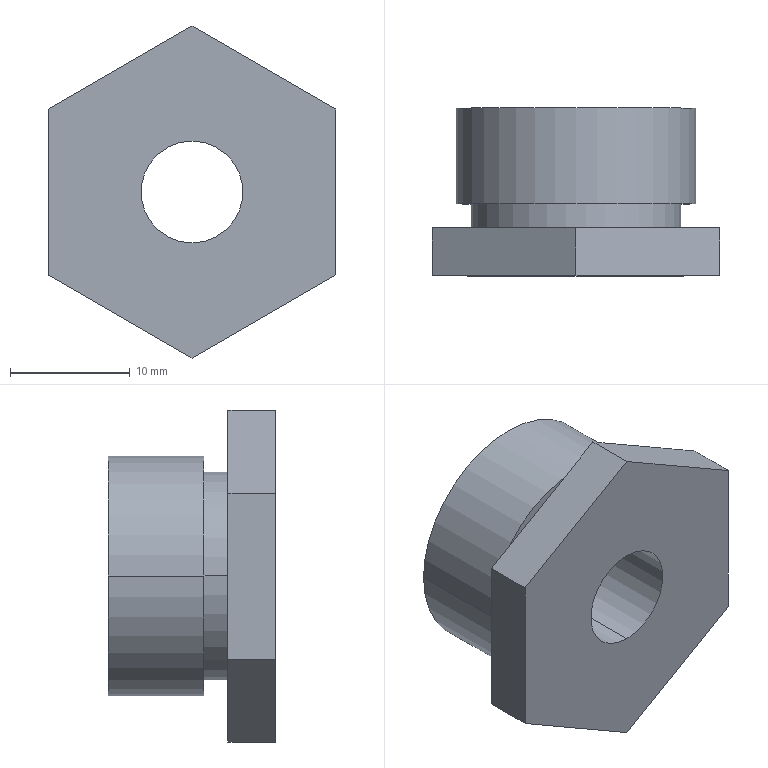Part | STEP file | Screen clamp lock bolt 2 | 1 solid | 16 faces | box 24 x 14 x 27.713 mm | volume 4195 mm3 | plane 10 | cylinder 6 | commonest cylinder face diameters 8.5 x2 17.5 x2 20 x2
STEP:
#1=CARTESIAN_POINT('',(-327.873,-1228.134,-13238.29));
#2=VERTEX_POINT('',#1);
#3=CARTESIAN_POINT('',(-310.373,-1228.134,-13238.29));
#4=VERTEX_POINT('',#3);
#5=CARTESIAN_POINT('',(-319.123,-1228.134,-13238.29));
#6=DIRECTION('',(0.,1.,0.));
#7=DIRECTION('',(-1.,0.,0.));
#8=AXIS2_PLACEMENT_3D('',#5,#6,#7);
#9=CIRCLE('',#8,8.75);
#10=EDGE_CURVE('',#2,#4,#9,.T.);
#11=ORIENTED_EDGE('',*,*,#10,.F.);
#12=CARTESIAN_POINT('',(-327.873,-1230.134,-13238.29));
#13=VERTEX_POINT('',#12);
#14=CARTESIAN_POINT('',(-327.873,-1228.134,-13238.29));
#15=DIRECTION('',(0.,-1.,0.));
#16=VECTOR('',#15,1000.);
#17=LINE('',#14,#16);
#18=EDGE_CURVE('',#2,#13,#17,.T.);
#19=ORIENTED_EDGE('',*,*,#18,.T.);
#20=CARTESIAN_POINT('',(-310.373,-1230.134,-13238.29));
#21=VERTEX_POINT('',#20);
#22=CARTESIAN_POINT('',(-319.123,-1230.134,-13238.29));
#23=DIRECTION('',(0.,1.,0.));
#24=DIRECTION('',(-1.,0.,0.));
#25=AXIS2_PLACEMENT_3D('',#22,#23,#24);
#26=CIRCLE('',#25,8.75);
#27=EDGE_CURVE('',#13,#21,#26,.T.);
#28=ORIENTED_EDGE('',*,*,#27,.T.);
#29=CARTESIAN_POINT('',(-310.373,-1228.134,-13238.29));
#30=DIRECTION('',(0.,-1.,0.));
#31=VECTOR('',#30,1000.);
#32=LINE('',#29,#31);
#33=EDGE_CURVE('',#4,#21,#32,.T.);
#34=ORIENTED_EDGE('',*,*,#33,.F.);
#35=EDGE_LOOP('',(#11,#19,#28,#34));
#36=FACE_OUTER_BOUND('',#35,.T.);
#37=CARTESIAN_POINT('',(-319.123,-1228.134,-13238.29));
#38=DIRECTION('',(0.,-1.,0.));
#39=DIRECTION('',(1.,0.,0.));
#40=AXIS2_PLACEMENT_3D('',#37,#38,#39);
#41=CYLINDRICAL_SURFACE('',#40,8.75);
#42=ADVANCED_FACE('',(#36),#41,.T.);
#43=CARTESIAN_POINT('',(-319.123,-1234.134,-13242.54));
#44=VERTEX_POINT('',#43);
#45=CARTESIAN_POINT('',(-319.123,-1234.134,-13234.04));
#46=VERTEX_POINT('',#45);
#47=CARTESIAN_POINT('',(-319.123,-1234.134,-13238.29));
#48=DIRECTION('',(0.,1.,0.));
#49=DIRECTION('',(0.,0.,1.));
#50=AXIS2_PLACEMENT_3D('',#47,#48,#49);
#51=CIRCLE('',#50,4.25);
#52=EDGE_CURVE('',#44,#46,#51,.T.);
#53=ORIENTED_EDGE('',*,*,#52,.F.);
#54=CARTESIAN_POINT('',(-319.123,-1220.134,-13242.54));
#55=VERTEX_POINT('',#54);
#56=CARTESIAN_POINT('',(-319.123,-1220.134,-13242.54));
#57=DIRECTION('',(0.,1.,0.));
#58=VECTOR('',#57,1000.);
#59=LINE('',#56,#58);
#60=EDGE_CURVE('',#44,#55,#59,.T.);
#61=ORIENTED_EDGE('',*,*,#60,.T.);
#62=CARTESIAN_POINT('',(-319.123,-1220.134,-13234.04));
#63=VERTEX_POINT('',#62);
#64=CARTESIAN_POINT('',(-319.123,-1220.134,-13238.29));
#65=DIRECTION('',(0.,1.,0.));
#66=DIRECTION('',(0.,0.,1.));
#67=AXIS2_PLACEMENT_3D('',#64,#65,#66);
#68=CIRCLE('',#67,4.25);
#69=EDGE_CURVE('',#55,#63,#68,.T.);
#70=ORIENTED_EDGE('',*,*,#69,.T.);
#71=CARTESIAN_POINT('',(-319.123,-1220.134,-13234.04));
#72=DIRECTION('',(0.,1.,0.));
#73=VECTOR('',#72,1000.);
#74=LINE('',#71,#73);
#75=EDGE_CURVE('',#46,#63,#74,.T.);
#76=ORIENTED_EDGE('',*,*,#75,.F.);
#77=EDGE_LOOP('',(#53,#61,#70,#76));
#78=FACE_OUTER_BOUND('',#77,.T.);
#79=CARTESIAN_POINT('',(-319.123,-1220.134,-13238.29));
#80=DIRECTION('',(0.,1.,0.));
#81=DIRECTION('',(0.,0.,1.));
#82=AXIS2_PLACEMENT_3D('',#79,#80,#81);
#83=CYLINDRICAL_SURFACE('',#82,4.25);
#84=ADVANCED_FACE('',(#78),#83,.F.);
#85=CARTESIAN_POINT('',(-309.123,-1220.134,-13238.29));
#86=VERTEX_POINT('',#85);
#87=CARTESIAN_POINT('',(-329.123,-1220.134,-13238.29));
#88=VERTEX_POINT('',#87);
#89=CARTESIAN_POINT('',(-319.123,-1220.134,-13238.29));
#90=DIRECTION('',(0.,-1.,0.));
#91=DIRECTION('',(1.,0.,0.));
#92=AXIS2_PLACEMENT_3D('',#89,#90,#91);
#93=CIRCLE('',#92,10.);
#94=EDGE_CURVE('',#86,#88,#93,.T.);
#95=ORIENTED_EDGE('',*,*,#94,.T.);
#96=CARTESIAN_POINT('',(-329.123,-1228.134,-13238.29));
#97=VERTEX_POINT('',#96);
#98=CARTESIAN_POINT('',(-329.123,-1220.134,-13238.29));
#99=DIRECTION('',(0.,-1.,0.));
#100=VECTOR('',#99,1000.);
#101=LINE('',#98,#100);
#102=EDGE_CURVE('',#88,#97,#101,.T.);
#103=ORIENTED_EDGE('',*,*,#102,.T.);
#104=CARTESIAN_POINT('',(-309.123,-1228.134,-13238.29));
#105=VERTEX_POINT('',#104);
#106=CARTESIAN_POINT('',(-319.123,-1228.134,-13238.29));
#107=DIRECTION('',(0.,1.,0.));
#108=DIRECTION('',(-1.,0.,0.));
#109=AXIS2_PLACEMENT_3D('',#106,#107,#108);
#110=CIRCLE('',#109,10.);
#111=EDGE_CURVE('',#97,#105,#110,.T.);
#112=ORIENTED_EDGE('',*,*,#111,.T.);
#113=CARTESIAN_POINT('',(-309.123,-1220.134,-13238.29));
#114=DIRECTION('',(0.,-1.,0.));
#115=VECTOR('',#114,1000.);
#116=LINE('',#113,#115);
#117=EDGE_CURVE('',#86,#105,#116,.T.);
#118=ORIENTED_EDGE('',*,*,#117,.F.);
#119=EDGE_LOOP('',(#95,#103,#112,#118));
#120=FACE_OUTER_BOUND('',#119,.T.);
#121=CARTESIAN_POINT('',(-319.123,-1220.134,-13238.29));
#122=DIRECTION('',(0.,-1.,0.));
#123=DIRECTION('',(1.,0.,0.));
#124=AXIS2_PLACEMENT_3D('',#121,#122,#123);
#125=CYLINDRICAL_SURFACE('',#124,10.);
#126=ADVANCED_FACE('',(#120),#125,.T.);
#127=ORIENTED_EDGE('',*,*,#102,.F.);
#128=CARTESIAN_POINT('',(-319.123,-1220.134,-13238.29));
#129=DIRECTION('',(0.,-1.,0.));
#130=DIRECTION('',(1.,0.,0.));
#131=AXIS2_PLACEMENT_3D('',#128,#129,#130);
#132=CIRCLE('',#131,10.);
#133=EDGE_CURVE('',#88,#86,#132,.T.);
#134=ORIENTED_EDGE('',*,*,#133,.T.);
#135=ORIENTED_EDGE('',*,*,#117,.T.);
#136=CARTESIAN_POINT('',(-319.123,-1228.134,-13238.29));
#137=DIRECTION('',(0.,1.,0.));
#138=DIRECTION('',(-1.,0.,0.));
#139=AXIS2_PLACEMENT_3D('',#136,#137,#138);
#140=CIRCLE('',#139,10.);
#141=EDGE_CURVE('',#105,#97,#140,.T.);
#142=ORIENTED_EDGE('',*,*,#141,.T.);
#143=EDGE_LOOP('',(#127,#134,#135,#142));
#144=FACE_OUTER_BOUND('',#143,.T.);
#145=CARTESIAN_POINT('',(-319.123,-1220.134,-13238.29));
#146=DIRECTION('',(0.,-1.,0.));
#147=DIRECTION('',(1.,0.,0.));
#148=AXIS2_PLACEMENT_3D('',#145,#146,#147);
#149=CYLINDRICAL_SURFACE('',#148,10.);
#150=ADVANCED_FACE('',(#144),#149,.T.);
#151=CARTESIAN_POINT('',(-319.123,-1220.134,-13238.29));
#152=DIRECTION('',(0.,1.,0.));
#153=DIRECTION('',(0.,0.,1.));
#154=AXIS2_PLACEMENT_3D('',#151,#152,#153);
#155=CIRCLE('',#154,4.25);
#156=EDGE_CURVE('',#63,#55,#155,.T.);
#157=ORIENTED_EDGE('',*,*,#156,.F.);
#158=ORIENTED_EDGE('',*,*,#69,.F.);
#159=EDGE_LOOP('',(#157,#158));
#160=FACE_BOUND('',#159,.T.);
#161=ORIENTED_EDGE('',*,*,#94,.F.);
#162=ORIENTED_EDGE('',*,*,#133,.F.);
#163=EDGE_LOOP('',(#161,#162));
#164=FACE_OUTER_BOUND('',#163,.T.);
#165=CARTESIAN_POINT('',(-319.123,-1220.134,-13238.29));
#166=DIRECTION('',(0.,-1.,0.));
#167=DIRECTION('',(1.,0.,0.));
#168=AXIS2_PLACEMENT_3D('',#165,#166,#167);
#169=PLANE('',#168);
#170=ADVANCED_FACE('',(#160,#164),#169,.F.);
#171=CARTESIAN_POINT('',(-307.123,-1230.134,-13231.361));
#172=VERTEX_POINT('',#171);
#173=CARTESIAN_POINT('',(-319.123,-1230.134,-13224.433));
#174=VERTEX_POINT('',#173);
#175=CARTESIAN_POINT('',(-307.123,-1230.134,-13231.361));
#176=DIRECTION('',(-0.866,0.,0.5));
#177=VECTOR('',#176,1000.);
#178=LINE('',#175,#177);
#179=EDGE_CURVE('',#172,#174,#178,.T.);
#180=ORIENTED_EDGE('',*,*,#179,.T.);
#181=CARTESIAN_POINT('',(-319.123,-1234.134,-13224.433));
#182=VERTEX_POINT('',#181);
#183=CARTESIAN_POINT('',(-319.123,-1234.134,-13224.433));
#184=DIRECTION('',(0.,1.,0.));
#185=VECTOR('',#184,1000.);
#186=LINE('',#183,#185);
#187=EDGE_CURVE('',#182,#174,#186,.T.);
#188=ORIENTED_EDGE('',*,*,#187,.F.);
#189=CARTESIAN_POINT('',(-307.123,-1234.134,-13231.361));
#190=VERTEX_POINT('',#189);
#191=CARTESIAN_POINT('',(-307.123,-1234.134,-13231.361));
#192=DIRECTION('',(-0.866,0.,0.5));
#193=VECTOR('',#192,1000.);
#194=LINE('',#191,#193);
#195=EDGE_CURVE('',#190,#182,#194,.T.);
#196=ORIENTED_EDGE('',*,*,#195,.F.);
#197=CARTESIAN_POINT('',(-307.123,-1234.134,-13231.361));
#198=DIRECTION('',(0.,1.,0.));
#199=VECTOR('',#198,1000.);
#200=LINE('',#197,#199);
#201=EDGE_CURVE('',#190,#172,#200,.T.);
#202=ORIENTED_EDGE('',*,*,#201,.T.);
#203=EDGE_LOOP('',(#180,#188,#196,#202));
#204=FACE_OUTER_BOUND('',#203,.T.);
#205=CARTESIAN_POINT('',(-307.123,-1234.134,-13231.361));
#206=DIRECTION('',(-0.5,0.,-0.866));
#207=DIRECTION('',(-0.866,0.,0.5));
#208=AXIS2_PLACEMENT_3D('',#205,#206,#207);
#209=PLANE('',#208);
#210=ADVANCED_FACE('',(#204),#209,.F.);
#211=CARTESIAN_POINT('',(-331.123,-1230.134,-13231.361));
#212=VERTEX_POINT('',#211);
#213=CARTESIAN_POINT('',(-319.123,-1230.134,-13224.433));
#214=DIRECTION('',(-0.866,0.,-0.5));
#215=VECTOR('',#214,1000.);
#216=LINE('',#213,#215);
#217=EDGE_CURVE('',#174,#212,#216,.T.);
#218=ORIENTED_EDGE('',*,*,#217,.T.);
#219=CARTESIAN_POINT('',(-331.123,-1234.134,-13231.361));
#220=VERTEX_POINT('',#219);
#221=CARTESIAN_POINT('',(-331.123,-1234.134,-13231.361));
#222=DIRECTION('',(0.,1.,0.));
#223=VECTOR('',#222,1000.);
#224=LINE('',#221,#223);
#225=EDGE_CURVE('',#220,#212,#224,.T.);
#226=ORIENTED_EDGE('',*,*,#225,.F.);
#227=CARTESIAN_POINT('',(-319.123,-1234.134,-13224.433));
#228=DIRECTION('',(-0.866,0.,-0.5));
#229=VECTOR('',#228,1000.);
#230=LINE('',#227,#229);
#231=EDGE_CURVE('',#182,#220,#230,.T.);
#232=ORIENTED_EDGE('',*,*,#231,.F.);
#233=ORIENTED_EDGE('',*,*,#187,.T.);
#234=EDGE_LOOP('',(#218,#226,#232,#233));
#235=FACE_OUTER_BOUND('',#234,.T.);
#236=CARTESIAN_POINT('',(-319.123,-1234.134,-13224.433));
#237=DIRECTION('',(0.5,0.,-0.866));
#238=DIRECTION('',(-0.866,0.,-0.5));
#239=AXIS2_PLACEMENT_3D('',#236,#237,#238);
#240=PLANE('',#239);
#241=ADVANCED_FACE('',(#235),#240,.F.);
#242=CARTESIAN_POINT('',(-331.122,-1230.134,-13245.218));
#243=VERTEX_POINT('',#242);
#244=CARTESIAN_POINT('',(-331.123,-1230.134,-13231.361));
#245=DIRECTION('',(0.000004464,0.,-1.));
#246=VECTOR('',#245,1000.);
#247=LINE('',#244,#246);
#248=EDGE_CURVE('',#212,#243,#247,.T.);
#249=ORIENTED_EDGE('',*,*,#248,.T.);
#250=CARTESIAN_POINT('',(-331.122,-1234.134,-13245.218));
#251=VERTEX_POINT('',#250);
#252=CARTESIAN_POINT('',(-331.122,-1234.134,-13245.218));
#253=DIRECTION('',(0.,1.,0.));
#254=VECTOR('',#253,1000.);
#255=LINE('',#252,#254);
#256=EDGE_CURVE('',#251,#243,#255,.T.);
#257=ORIENTED_EDGE('',*,*,#256,.F.);
#258=CARTESIAN_POINT('',(-331.123,-1234.134,-13231.361));
#259=DIRECTION('',(0.000004464,0.,-1.));
#260=VECTOR('',#259,1000.);
#261=LINE('',#258,#260);
#262=EDGE_CURVE('',#220,#251,#261,.T.);
#263=ORIENTED_EDGE('',*,*,#262,.F.);
#264=ORIENTED_EDGE('',*,*,#225,.T.);
#265=EDGE_LOOP('',(#249,#257,#263,#264));
#266=FACE_OUTER_BOUND('',#265,.T.);
#267=CARTESIAN_POINT('',(-331.123,-1234.134,-13231.361));
#268=DIRECTION('',(1.,0.,0.000004464));
#269=DIRECTION('',(0.000004464,0.,-1.));
#270=AXIS2_PLACEMENT_3D('',#267,#268,#269);
#271=PLANE('',#270);
#272=ADVANCED_FACE('',(#266),#271,.F.);
#273=CARTESIAN_POINT('',(-319.122,-1230.134,-13252.146));
#274=VERTEX_POINT('',#273);
#275=CARTESIAN_POINT('',(-331.122,-1230.134,-13245.218));
#276=DIRECTION('',(0.866,0.,-0.5));
#277=VECTOR('',#276,1000.);
#278=LINE('',#275,#277);
#279=EDGE_CURVE('',#243,#274,#278,.T.);
#280=ORIENTED_EDGE('',*,*,#279,.T.);
#281=CARTESIAN_POINT('',(-319.122,-1234.134,-13252.146));
#282=VERTEX_POINT('',#281);
#283=CARTESIAN_POINT('',(-319.122,-1234.134,-13252.146));
#284=DIRECTION('',(0.,1.,0.));
#285=VECTOR('',#284,1000.);
#286=LINE('',#283,#285);
#287=EDGE_CURVE('',#282,#274,#286,.T.);
#288=ORIENTED_EDGE('',*,*,#287,.F.);
#289=CARTESIAN_POINT('',(-331.122,-1234.134,-13245.218));
#290=DIRECTION('',(0.866,0.,-0.5));
#291=VECTOR('',#290,1000.);
#292=LINE('',#289,#291);
#293=EDGE_CURVE('',#251,#282,#292,.T.);
#294=ORIENTED_EDGE('',*,*,#293,.F.);
#295=ORIENTED_EDGE('',*,*,#256,.T.);
#296=EDGE_LOOP('',(#280,#288,#294,#295));
#297=FACE_OUTER_BOUND('',#296,.T.);
#298=CARTESIAN_POINT('',(-331.122,-1234.134,-13245.218));
#299=DIRECTION('',(0.5,0.,0.866));
#300=DIRECTION('',(0.866,0.,-0.5));
#301=AXIS2_PLACEMENT_3D('',#298,#299,#300);
#302=PLANE('',#301);
#303=ADVANCED_FACE('',(#297),#302,.F.);
#304=CARTESIAN_POINT('',(-307.122,-1230.134,-13245.218));
#305=VERTEX_POINT('',#304);
#306=CARTESIAN_POINT('',(-319.122,-1230.134,-13252.146));
#307=DIRECTION('',(0.866,0.,0.5));
#308=VECTOR('',#307,1000.);
#309=LINE('',#306,#308);
#310=EDGE_CURVE('',#274,#305,#309,.T.);
#311=ORIENTED_EDGE('',*,*,#310,.T.);
#312=CARTESIAN_POINT('',(-307.122,-1234.134,-13245.218));
#313=VERTEX_POINT('',#312);
#314=CARTESIAN_POINT('',(-307.122,-1234.134,-13245.218));
#315=DIRECTION('',(0.,1.,0.));
#316=VECTOR('',#315,1000.);
#317=LINE('',#314,#316);
#318=EDGE_CURVE('',#313,#305,#317,.T.);
#319=ORIENTED_EDGE('',*,*,#318,.F.);
#320=CARTESIAN_POINT('',(-319.122,-1234.134,-13252.146));
#321=DIRECTION('',(0.866,0.,0.5));
#322=VECTOR('',#321,1000.);
#323=LINE('',#320,#322);
#324=EDGE_CURVE('',#282,#313,#323,.T.);
#325=ORIENTED_EDGE('',*,*,#324,.F.);
#326=ORIENTED_EDGE('',*,*,#287,.T.);
#327=EDGE_LOOP('',(#311,#319,#325,#326));
#328=FACE_OUTER_BOUND('',#327,.T.);
#329=CARTESIAN_POINT('',(-319.122,-1234.134,-13252.146));
#330=DIRECTION('',(-0.5,0.,0.866));
#331=DIRECTION('',(0.866,0.,0.5));
#332=AXIS2_PLACEMENT_3D('',#329,#330,#331);
#333=PLANE('',#332);
#334=ADVANCED_FACE('',(#328),#333,.F.);
#335=CARTESIAN_POINT('',(-307.122,-1230.134,-13245.218));
#336=DIRECTION('',(-0.000004464,0.,1.));
#337=VECTOR('',#336,1000.);
#338=LINE('',#335,#337);
#339=EDGE_CURVE('',#305,#172,#338,.T.);
#340=ORIENTED_EDGE('',*,*,#339,.T.);
#341=ORIENTED_EDGE('',*,*,#201,.F.);
#342=CARTESIAN_POINT('',(-307.122,-1234.134,-13245.218));
#343=DIRECTION('',(-0.000004464,0.,1.));
#344=VECTOR('',#343,1000.);
#345=LINE('',#342,#344);
#346=EDGE_CURVE('',#313,#190,#345,.T.);
#347=ORIENTED_EDGE('',*,*,#346,.F.);
#348=ORIENTED_EDGE('',*,*,#318,.T.);
#349=EDGE_LOOP('',(#340,#341,#347,#348));
#350=FACE_OUTER_BOUND('',#349,.T.);
#351=CARTESIAN_POINT('',(-307.122,-1234.134,-13245.218));
#352=DIRECTION('',(-1.,0.,-0.000004464));
#353=DIRECTION('',(-0.000004464,0.,1.));
#354=AXIS2_PLACEMENT_3D('',#351,#352,#353);
#355=PLANE('',#354);
#356=ADVANCED_FACE('',(#350),#355,.F.);
#357=CARTESIAN_POINT('',(-319.123,-1234.134,-13238.29));
#358=DIRECTION('',(0.,1.,0.));
#359=DIRECTION('',(0.,0.,1.));
#360=AXIS2_PLACEMENT_3D('',#357,#358,#359);
#361=CIRCLE('',#360,4.25);
#362=EDGE_CURVE('',#46,#44,#361,.T.);
#363=ORIENTED_EDGE('',*,*,#362,.T.);
#364=ORIENTED_EDGE('',*,*,#52,.T.);
#365=EDGE_LOOP('',(#363,#364));
#366=FACE_BOUND('',#365,.T.);
#367=ORIENTED_EDGE('',*,*,#195,.T.);
#368=ORIENTED_EDGE('',*,*,#231,.T.);
#369=ORIENTED_EDGE('',*,*,#262,.T.);
#370=ORIENTED_EDGE('',*,*,#293,.T.);
#371=ORIENTED_EDGE('',*,*,#324,.T.);
#372=ORIENTED_EDGE('',*,*,#346,.T.);
#373=EDGE_LOOP('',(#367,#368,#369,#370,#371,#372));
#374=FACE_OUTER_BOUND('',#373,.T.);
#375=CARTESIAN_POINT('',(-319.123,-1234.134,-13224.433));
#376=DIRECTION('',(0.,-1.,0.));
#377=DIRECTION('',(1.,0.,0.));
#378=AXIS2_PLACEMENT_3D('',#375,#376,#377);
#379=PLANE('',#378);
#380=ADVANCED_FACE('',(#366,#374),#379,.T.);
#381=ORIENTED_EDGE('',*,*,#179,.F.);
#382=ORIENTED_EDGE('',*,*,#339,.F.);
#383=ORIENTED_EDGE('',*,*,#310,.F.);
#384=ORIENTED_EDGE('',*,*,#279,.F.);
#385=ORIENTED_EDGE('',*,*,#248,.F.);
#386=ORIENTED_EDGE('',*,*,#217,.F.);
#387=EDGE_LOOP('',(#381,#382,#383,#384,#385,#386));
#388=FACE_OUTER_BOUND('',#387,.T.);
#389=CARTESIAN_POINT('',(-319.123,-1230.134,-13238.29));
#390=DIRECTION('',(0.,1.,0.));
#391=DIRECTION('',(-1.,0.,0.));
#392=AXIS2_PLACEMENT_3D('',#389,#390,#391);
#393=CIRCLE('',#392,8.75);
#394=EDGE_CURVE('',#21,#13,#393,.T.);
#395=ORIENTED_EDGE('',*,*,#394,.F.);
#396=ORIENTED_EDGE('',*,*,#27,.F.);
#397=EDGE_LOOP('',(#395,#396));
#398=FACE_BOUND('',#397,.T.);
#399=CARTESIAN_POINT('',(-319.123,-1230.134,-13224.433));
#400=DIRECTION('',(0.,-1.,0.));
#401=DIRECTION('',(1.,0.,0.));
#402=AXIS2_PLACEMENT_3D('',#399,#400,#401);
#403=PLANE('',#402);
#404=ADVANCED_FACE('',(#388,#398),#403,.F.);
#405=ORIENTED_EDGE('',*,*,#60,.F.);
#406=ORIENTED_EDGE('',*,*,#362,.F.);
#407=ORIENTED_EDGE('',*,*,#75,.T.);
#408=ORIENTED_EDGE('',*,*,#156,.T.);
#409=EDGE_LOOP('',(#405,#406,#407,#408));
#410=FACE_OUTER_BOUND('',#409,.T.);
#411=CARTESIAN_POINT('',(-319.123,-1220.134,-13238.29));
#412=DIRECTION('',(0.,1.,0.));
#413=DIRECTION('',(0.,0.,1.));
#414=AXIS2_PLACEMENT_3D('',#411,#412,#413);
#415=CYLINDRICAL_SURFACE('',#414,4.25);
#416=ADVANCED_FACE('',(#410),#415,.F.);
#417=ORIENTED_EDGE('',*,*,#141,.F.);
#418=ORIENTED_EDGE('',*,*,#111,.F.);
#419=EDGE_LOOP('',(#417,#418));
#420=FACE_OUTER_BOUND('',#419,.T.);
#421=CARTESIAN_POINT('',(-319.123,-1228.134,-13238.29));
#422=DIRECTION('',(0.,1.,0.));
#423=DIRECTION('',(-1.,0.,0.));
#424=AXIS2_PLACEMENT_3D('',#421,#422,#423);
#425=CIRCLE('',#424,8.75);
#426=EDGE_CURVE('',#4,#2,#425,.T.);
#427=ORIENTED_EDGE('',*,*,#426,.T.);
#428=ORIENTED_EDGE('',*,*,#10,.T.);
#429=EDGE_LOOP('',(#427,#428));
#430=FACE_BOUND('',#429,.T.);
#431=CARTESIAN_POINT('',(-319.123,-1228.134,-13238.29));
#432=DIRECTION('',(0.,1.,0.));
#433=DIRECTION('',(-1.,0.,0.));
#434=AXIS2_PLACEMENT_3D('',#431,#432,#433);
#435=PLANE('',#434);
#436=ADVANCED_FACE('',(#420,#430),#435,.F.);
#437=ORIENTED_EDGE('',*,*,#18,.F.);
#438=ORIENTED_EDGE('',*,*,#426,.F.);
#439=ORIENTED_EDGE('',*,*,#33,.T.);
#440=ORIENTED_EDGE('',*,*,#394,.T.);
#441=EDGE_LOOP('',(#437,#438,#439,#440));
#442=FACE_OUTER_BOUND('',#441,.T.);
#443=CARTESIAN_POINT('',(-319.123,-1228.134,-13238.29));
#444=DIRECTION('',(0.,-1.,0.));
#445=DIRECTION('',(1.,0.,0.));
#446=AXIS2_PLACEMENT_3D('',#443,#444,#445);
#447=CYLINDRICAL_SURFACE('',#446,8.75);
#448=ADVANCED_FACE('',(#442),#447,.T.);
#449=CLOSED_SHELL('',(#42,#84,#126,#150,#170,#210,#241,#272,#303,#334,#356,#380,#404,#416,#436,#448));
#450=MANIFOLD_SOLID_BREP('',#449);
#451=CARTESIAN_POINT('',(0.,0.,0.));
#452=DIRECTION('',(0.,0.,1.));
#453=DIRECTION('',(1.,0.,0.));
#454=AXIS2_PLACEMENT_3D('',#451,#452,#453);
#455=(LENGTH_UNIT()NAMED_UNIT(*)SI_UNIT(.MILLI.,.METRE.));
#456=UNCERTAINTY_MEASURE_WITH_UNIT(LENGTH_MEASURE(0.00001),#455,'','');
#457=(NAMED_UNIT(*)PLANE_ANGLE_UNIT()SI_UNIT($,.RADIAN.));
#458=(NAMED_UNIT(*)SI_UNIT($,.STERADIAN.)SOLID_ANGLE_UNIT());
#459=(GEOMETRIC_REPRESENTATION_CONTEXT(3)GLOBAL_UNCERTAINTY_ASSIGNED_CONTEXT((#456))GLOBAL_UNIT_ASSIGNED_CONTEXT((#455,#457,#458))REPRESENTATION_CONTEXT('',''));
#460=ADVANCED_BREP_SHAPE_REPRESENTATION('',(#450,#454),#459);